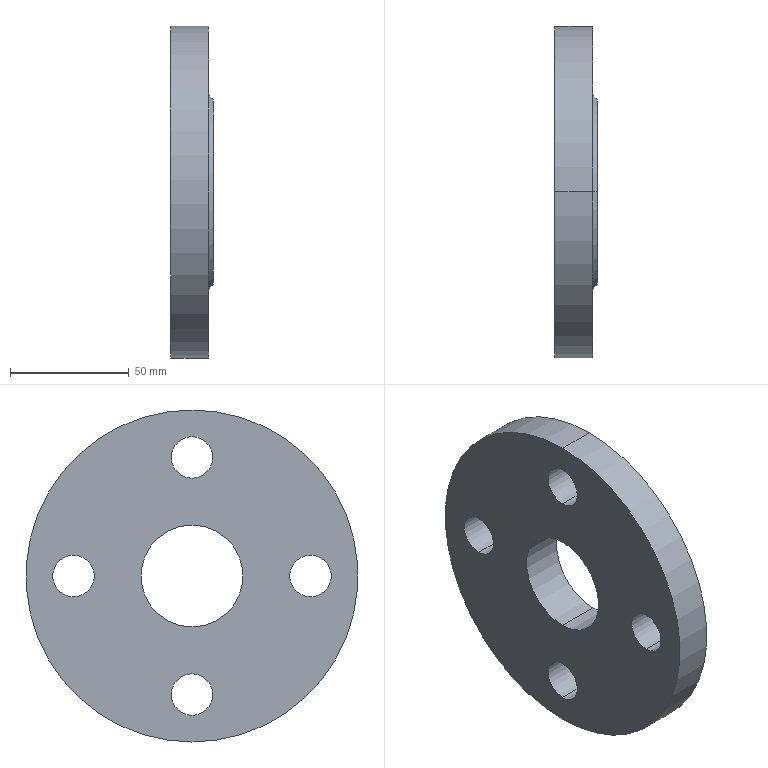Part | SolidWorks | features ICE 1, Revolution 1 | 1 solid | 17 faces | box 18 x 140 x 140 mm | volume 214823 mm3 | cylinder 12 | plane 3 | cone 2 | commonest cylinder face diameters 17.5 x8 43 x2 140 x2
STEP:
#1=CARTESIAN_POINT('',(0.,50.,8.75));
#2=VERTEX_POINT('',#1);
#3=CARTESIAN_POINT('',(0.,50.,-8.75));
#4=VERTEX_POINT('',#3);
#5=CARTESIAN_POINT('',(0.,50.,0.));
#6=DIRECTION('',(1.,0.,0.));
#7=DIRECTION('',(0.,0.,-1.));
#8=AXIS2_PLACEMENT_3D('',#5,#6,#7);
#9=CIRCLE('',#8,8.75);
#10=EDGE_CURVE('',#2,#4,#9,.T.);
#11=ORIENTED_EDGE('',*,*,#10,.F.);
#12=CARTESIAN_POINT('',(16.,50.,8.75));
#13=VERTEX_POINT('',#12);
#14=CARTESIAN_POINT('',(0.,50.,8.75));
#15=DIRECTION('',(1.,0.,0.));
#16=VECTOR('',#15,1000.);
#17=LINE('',#14,#16);
#18=EDGE_CURVE('',#2,#13,#17,.T.);
#19=ORIENTED_EDGE('',*,*,#18,.T.);
#20=CARTESIAN_POINT('',(16.,50.,-8.75));
#21=VERTEX_POINT('',#20);
#22=CARTESIAN_POINT('',(16.,50.,0.));
#23=DIRECTION('',(-1.,0.,0.));
#24=DIRECTION('',(0.,0.,1.));
#25=AXIS2_PLACEMENT_3D('',#22,#23,#24);
#26=CIRCLE('',#25,8.75);
#27=EDGE_CURVE('',#21,#13,#26,.T.);
#28=ORIENTED_EDGE('',*,*,#27,.F.);
#29=CARTESIAN_POINT('',(0.,50.,-8.75));
#30=DIRECTION('',(1.,0.,0.));
#31=VECTOR('',#30,1000.);
#32=LINE('',#29,#31);
#33=EDGE_CURVE('',#4,#21,#32,.T.);
#34=ORIENTED_EDGE('',*,*,#33,.F.);
#35=EDGE_LOOP('',(#11,#19,#28,#34));
#36=FACE_OUTER_BOUND('',#35,.T.);
#37=CARTESIAN_POINT('',(0.,50.,0.));
#38=DIRECTION('',(1.,0.,0.));
#39=DIRECTION('',(0.,0.,-1.));
#40=AXIS2_PLACEMENT_3D('',#37,#38,#39);
#41=CYLINDRICAL_SURFACE('',#40,8.75);
#42=ADVANCED_FACE('',(#36),#41,.F.);
#43=CARTESIAN_POINT('',(0.,0.,-41.25));
#44=VERTEX_POINT('',#43);
#45=CARTESIAN_POINT('',(0.,0.,-58.75));
#46=VERTEX_POINT('',#45);
#47=CARTESIAN_POINT('',(0.,0.,-50.));
#48=DIRECTION('',(1.,0.,0.));
#49=DIRECTION('',(0.,0.,-1.));
#50=AXIS2_PLACEMENT_3D('',#47,#48,#49);
#51=CIRCLE('',#50,8.75);
#52=EDGE_CURVE('',#44,#46,#51,.T.);
#53=ORIENTED_EDGE('',*,*,#52,.F.);
#54=CARTESIAN_POINT('',(16.,0.,-41.25));
#55=VERTEX_POINT('',#54);
#56=CARTESIAN_POINT('',(0.,0.,-41.25));
#57=DIRECTION('',(1.,0.,0.));
#58=VECTOR('',#57,1000.);
#59=LINE('',#56,#58);
#60=EDGE_CURVE('',#44,#55,#59,.T.);
#61=ORIENTED_EDGE('',*,*,#60,.T.);
#62=CARTESIAN_POINT('',(16.,0.,-58.75));
#63=VERTEX_POINT('',#62);
#64=CARTESIAN_POINT('',(16.,0.,-50.));
#65=DIRECTION('',(-1.,0.,0.));
#66=DIRECTION('',(0.,0.,1.));
#67=AXIS2_PLACEMENT_3D('',#64,#65,#66);
#68=CIRCLE('',#67,8.75);
#69=EDGE_CURVE('',#63,#55,#68,.T.);
#70=ORIENTED_EDGE('',*,*,#69,.F.);
#71=CARTESIAN_POINT('',(0.,0.,-58.75));
#72=DIRECTION('',(1.,0.,0.));
#73=VECTOR('',#72,1000.);
#74=LINE('',#71,#73);
#75=EDGE_CURVE('',#46,#63,#74,.T.);
#76=ORIENTED_EDGE('',*,*,#75,.F.);
#77=EDGE_LOOP('',(#53,#61,#70,#76));
#78=FACE_OUTER_BOUND('',#77,.T.);
#79=CARTESIAN_POINT('',(0.,0.,-50.));
#80=DIRECTION('',(1.,0.,0.));
#81=DIRECTION('',(0.,0.,-1.));
#82=AXIS2_PLACEMENT_3D('',#79,#80,#81);
#83=CYLINDRICAL_SURFACE('',#82,8.75);
#84=ADVANCED_FACE('',(#78),#83,.F.);
#85=CARTESIAN_POINT('',(0.,-50.,8.75));
#86=VERTEX_POINT('',#85);
#87=CARTESIAN_POINT('',(0.,-50.,-8.75));
#88=VERTEX_POINT('',#87);
#89=CARTESIAN_POINT('',(0.,-50.,0.));
#90=DIRECTION('',(1.,0.,0.));
#91=DIRECTION('',(0.,0.,-1.));
#92=AXIS2_PLACEMENT_3D('',#89,#90,#91);
#93=CIRCLE('',#92,8.75);
#94=EDGE_CURVE('',#86,#88,#93,.T.);
#95=ORIENTED_EDGE('',*,*,#94,.F.);
#96=CARTESIAN_POINT('',(16.,-50.,8.75));
#97=VERTEX_POINT('',#96);
#98=CARTESIAN_POINT('',(0.,-50.,8.75));
#99=DIRECTION('',(1.,0.,0.));
#100=VECTOR('',#99,1000.);
#101=LINE('',#98,#100);
#102=EDGE_CURVE('',#86,#97,#101,.T.);
#103=ORIENTED_EDGE('',*,*,#102,.T.);
#104=CARTESIAN_POINT('',(16.,-50.,-8.75));
#105=VERTEX_POINT('',#104);
#106=CARTESIAN_POINT('',(16.,-50.,0.));
#107=DIRECTION('',(-1.,0.,0.));
#108=DIRECTION('',(0.,0.,1.));
#109=AXIS2_PLACEMENT_3D('',#106,#107,#108);
#110=CIRCLE('',#109,8.75);
#111=EDGE_CURVE('',#105,#97,#110,.T.);
#112=ORIENTED_EDGE('',*,*,#111,.F.);
#113=CARTESIAN_POINT('',(0.,-50.,-8.75));
#114=DIRECTION('',(1.,0.,0.));
#115=VECTOR('',#114,1000.);
#116=LINE('',#113,#115);
#117=EDGE_CURVE('',#88,#105,#116,.T.);
#118=ORIENTED_EDGE('',*,*,#117,.F.);
#119=EDGE_LOOP('',(#95,#103,#112,#118));
#120=FACE_OUTER_BOUND('',#119,.T.);
#121=CARTESIAN_POINT('',(0.,-50.,0.));
#122=DIRECTION('',(1.,0.,0.));
#123=DIRECTION('',(0.,0.,-1.));
#124=AXIS2_PLACEMENT_3D('',#121,#122,#123);
#125=CYLINDRICAL_SURFACE('',#124,8.75);
#126=ADVANCED_FACE('',(#120),#125,.F.);
#127=CARTESIAN_POINT('',(0.,0.,58.75));
#128=VERTEX_POINT('',#127);
#129=CARTESIAN_POINT('',(0.,0.,41.25));
#130=VERTEX_POINT('',#129);
#131=CARTESIAN_POINT('',(0.,0.,50.));
#132=DIRECTION('',(1.,0.,0.));
#133=DIRECTION('',(0.,0.,-1.));
#134=AXIS2_PLACEMENT_3D('',#131,#132,#133);
#135=CIRCLE('',#134,8.75);
#136=EDGE_CURVE('',#128,#130,#135,.T.);
#137=ORIENTED_EDGE('',*,*,#136,.F.);
#138=CARTESIAN_POINT('',(16.,0.,58.75));
#139=VERTEX_POINT('',#138);
#140=CARTESIAN_POINT('',(0.,0.,58.75));
#141=DIRECTION('',(1.,0.,0.));
#142=VECTOR('',#141,1000.);
#143=LINE('',#140,#142);
#144=EDGE_CURVE('',#128,#139,#143,.T.);
#145=ORIENTED_EDGE('',*,*,#144,.T.);
#146=CARTESIAN_POINT('',(16.,0.,41.25));
#147=VERTEX_POINT('',#146);
#148=CARTESIAN_POINT('',(16.,0.,50.));
#149=DIRECTION('',(-1.,0.,0.));
#150=DIRECTION('',(0.,0.,1.));
#151=AXIS2_PLACEMENT_3D('',#148,#149,#150);
#152=CIRCLE('',#151,8.75);
#153=EDGE_CURVE('',#147,#139,#152,.T.);
#154=ORIENTED_EDGE('',*,*,#153,.F.);
#155=CARTESIAN_POINT('',(0.,0.,41.25));
#156=DIRECTION('',(1.,0.,0.));
#157=VECTOR('',#156,1000.);
#158=LINE('',#155,#157);
#159=EDGE_CURVE('',#130,#147,#158,.T.);
#160=ORIENTED_EDGE('',*,*,#159,.F.);
#161=EDGE_LOOP('',(#137,#145,#154,#160));
#162=FACE_OUTER_BOUND('',#161,.T.);
#163=CARTESIAN_POINT('',(0.,0.,50.));
#164=DIRECTION('',(1.,0.,0.));
#165=DIRECTION('',(0.,0.,-1.));
#166=AXIS2_PLACEMENT_3D('',#163,#164,#165);
#167=CYLINDRICAL_SURFACE('',#166,8.75);
#168=ADVANCED_FACE('',(#162),#167,.F.);
#169=CARTESIAN_POINT('',(18.,0.,39.));
#170=VERTEX_POINT('',#169);
#171=CARTESIAN_POINT('',(18.,0.,-39.));
#172=VERTEX_POINT('',#171);
#173=CARTESIAN_POINT('',(18.,0.,0.));
#174=DIRECTION('',(-1.,0.,0.));
#175=DIRECTION('',(0.,0.,1.));
#176=AXIS2_PLACEMENT_3D('',#173,#174,#175);
#177=CIRCLE('',#176,39.);
#178=EDGE_CURVE('',#170,#172,#177,.T.);
#179=ORIENTED_EDGE('',*,*,#178,.T.);
#180=CARTESIAN_POINT('',(16.,0.,-41.));
#181=VERTEX_POINT('',#180);
#182=CARTESIAN_POINT('',(18.,0.,-39.));
#183=DIRECTION('',(-0.7071,0.,-0.7071));
#184=VECTOR('',#183,1000.);
#185=LINE('',#182,#184);
#186=EDGE_CURVE('',#172,#181,#185,.T.);
#187=ORIENTED_EDGE('',*,*,#186,.T.);
#188=CARTESIAN_POINT('',(16.,0.,41.));
#189=VERTEX_POINT('',#188);
#190=CARTESIAN_POINT('',(16.,0.,0.));
#191=DIRECTION('',(-1.,0.,0.));
#192=DIRECTION('',(0.,0.,1.));
#193=AXIS2_PLACEMENT_3D('',#190,#191,#192);
#194=CIRCLE('',#193,41.);
#195=EDGE_CURVE('',#189,#181,#194,.T.);
#196=ORIENTED_EDGE('',*,*,#195,.F.);
#197=CARTESIAN_POINT('',(18.,0.,39.));
#198=DIRECTION('',(-0.7071,0.,0.7071));
#199=VECTOR('',#198,1000.);
#200=LINE('',#197,#199);
#201=EDGE_CURVE('',#170,#189,#200,.T.);
#202=ORIENTED_EDGE('',*,*,#201,.F.);
#203=EDGE_LOOP('',(#179,#187,#196,#202));
#204=FACE_OUTER_BOUND('',#203,.T.);
#205=CARTESIAN_POINT('',(18.,0.,0.));
#206=DIRECTION('',(-1.,0.,0.));
#207=DIRECTION('',(0.,0.,1.));
#208=AXIS2_PLACEMENT_3D('',#205,#206,#207);
#209=CONICAL_SURFACE('',#208,39.,0.7854);
#210=ADVANCED_FACE('',(#204),#209,.T.);
#211=CARTESIAN_POINT('',(16.,0.,70.));
#212=VERTEX_POINT('',#211);
#213=CARTESIAN_POINT('',(16.,0.,-70.));
#214=VERTEX_POINT('',#213);
#215=CARTESIAN_POINT('',(16.,0.,0.));
#216=DIRECTION('',(-1.,0.,0.));
#217=DIRECTION('',(0.,0.,1.));
#218=AXIS2_PLACEMENT_3D('',#215,#216,#217);
#219=CIRCLE('',#218,70.);
#220=EDGE_CURVE('',#212,#214,#219,.T.);
#221=ORIENTED_EDGE('',*,*,#220,.T.);
#222=CARTESIAN_POINT('',(0.,0.,-70.));
#223=VERTEX_POINT('',#222);
#224=CARTESIAN_POINT('',(0.,0.,-70.));
#225=DIRECTION('',(-1.,0.,0.));
#226=VECTOR('',#225,1000.);
#227=LINE('',#224,#226);
#228=EDGE_CURVE('',#214,#223,#227,.T.);
#229=ORIENTED_EDGE('',*,*,#228,.T.);
#230=CARTESIAN_POINT('',(0.,0.,70.));
#231=VERTEX_POINT('',#230);
#232=CARTESIAN_POINT('',(0.,0.,0.));
#233=DIRECTION('',(-1.,0.,0.));
#234=DIRECTION('',(0.,0.,1.));
#235=AXIS2_PLACEMENT_3D('',#232,#233,#234);
#236=CIRCLE('',#235,70.);
#237=EDGE_CURVE('',#231,#223,#236,.T.);
#238=ORIENTED_EDGE('',*,*,#237,.F.);
#239=CARTESIAN_POINT('',(0.,0.,70.));
#240=DIRECTION('',(-1.,0.,0.));
#241=VECTOR('',#240,1000.);
#242=LINE('',#239,#241);
#243=EDGE_CURVE('',#212,#231,#242,.T.);
#244=ORIENTED_EDGE('',*,*,#243,.F.);
#245=EDGE_LOOP('',(#221,#229,#238,#244));
#246=FACE_OUTER_BOUND('',#245,.T.);
#247=CARTESIAN_POINT('',(0.,0.,0.));
#248=DIRECTION('',(-1.,0.,0.));
#249=DIRECTION('',(0.,0.,1.));
#250=AXIS2_PLACEMENT_3D('',#247,#248,#249);
#251=CYLINDRICAL_SURFACE('',#250,70.);
#252=ADVANCED_FACE('',(#246),#251,.T.);
#253=CARTESIAN_POINT('',(18.,0.,-21.5));
#254=VERTEX_POINT('',#253);
#255=CARTESIAN_POINT('',(18.,0.,21.5));
#256=VERTEX_POINT('',#255);
#257=CARTESIAN_POINT('',(18.,0.,0.));
#258=DIRECTION('',(-1.,0.,0.));
#259=DIRECTION('',(0.,0.,1.));
#260=AXIS2_PLACEMENT_3D('',#257,#258,#259);
#261=CIRCLE('',#260,21.5);
#262=EDGE_CURVE('',#254,#256,#261,.T.);
#263=ORIENTED_EDGE('',*,*,#262,.F.);
#264=CARTESIAN_POINT('',(0.,0.,-21.5));
#265=VERTEX_POINT('',#264);
#266=CARTESIAN_POINT('',(0.,0.,-21.5));
#267=DIRECTION('',(-1.,0.,0.));
#268=VECTOR('',#267,1000.);
#269=LINE('',#266,#268);
#270=EDGE_CURVE('',#254,#265,#269,.T.);
#271=ORIENTED_EDGE('',*,*,#270,.T.);
#272=CARTESIAN_POINT('',(0.,0.,21.5));
#273=VERTEX_POINT('',#272);
#274=CARTESIAN_POINT('',(0.,0.,0.));
#275=DIRECTION('',(-1.,0.,0.));
#276=DIRECTION('',(0.,0.,1.));
#277=AXIS2_PLACEMENT_3D('',#274,#275,#276);
#278=CIRCLE('',#277,21.5);
#279=EDGE_CURVE('',#265,#273,#278,.T.);
#280=ORIENTED_EDGE('',*,*,#279,.T.);
#281=CARTESIAN_POINT('',(0.,0.,21.5));
#282=DIRECTION('',(-1.,0.,0.));
#283=VECTOR('',#282,1000.);
#284=LINE('',#281,#283);
#285=EDGE_CURVE('',#256,#273,#284,.T.);
#286=ORIENTED_EDGE('',*,*,#285,.F.);
#287=EDGE_LOOP('',(#263,#271,#280,#286));
#288=FACE_OUTER_BOUND('',#287,.T.);
#289=CARTESIAN_POINT('',(0.,0.,0.));
#290=DIRECTION('',(-1.,0.,0.));
#291=DIRECTION('',(0.,0.,1.));
#292=AXIS2_PLACEMENT_3D('',#289,#290,#291);
#293=CYLINDRICAL_SURFACE('',#292,21.5);
#294=ADVANCED_FACE('',(#288),#293,.F.);
#295=ORIENTED_EDGE('',*,*,#270,.F.);
#296=CARTESIAN_POINT('',(18.,0.,0.));
#297=DIRECTION('',(-1.,0.,0.));
#298=DIRECTION('',(0.,0.,1.));
#299=AXIS2_PLACEMENT_3D('',#296,#297,#298);
#300=CIRCLE('',#299,21.5);
#301=EDGE_CURVE('',#256,#254,#300,.T.);
#302=ORIENTED_EDGE('',*,*,#301,.F.);
#303=ORIENTED_EDGE('',*,*,#285,.T.);
#304=CARTESIAN_POINT('',(0.,0.,0.));
#305=DIRECTION('',(-1.,0.,0.));
#306=DIRECTION('',(0.,0.,1.));
#307=AXIS2_PLACEMENT_3D('',#304,#305,#306);
#308=CIRCLE('',#307,21.5);
#309=EDGE_CURVE('',#273,#265,#308,.T.);
#310=ORIENTED_EDGE('',*,*,#309,.T.);
#311=EDGE_LOOP('',(#295,#302,#303,#310));
#312=FACE_OUTER_BOUND('',#311,.T.);
#313=CARTESIAN_POINT('',(0.,0.,0.));
#314=DIRECTION('',(-1.,0.,0.));
#315=DIRECTION('',(0.,0.,1.));
#316=AXIS2_PLACEMENT_3D('',#313,#314,#315);
#317=CYLINDRICAL_SURFACE('',#316,21.5);
#318=ADVANCED_FACE('',(#312),#317,.F.);
#319=CARTESIAN_POINT('',(0.,50.,0.));
#320=DIRECTION('',(1.,0.,0.));
#321=DIRECTION('',(0.,0.,-1.));
#322=AXIS2_PLACEMENT_3D('',#319,#320,#321);
#323=CIRCLE('',#322,8.75);
#324=EDGE_CURVE('',#4,#2,#323,.T.);
#325=ORIENTED_EDGE('',*,*,#324,.T.);
#326=ORIENTED_EDGE('',*,*,#10,.T.);
#327=EDGE_LOOP('',(#325,#326));
#328=FACE_BOUND('',#327,.T.);
#329=CARTESIAN_POINT('',(0.,0.,-50.));
#330=DIRECTION('',(1.,0.,0.));
#331=DIRECTION('',(0.,0.,-1.));
#332=AXIS2_PLACEMENT_3D('',#329,#330,#331);
#333=CIRCLE('',#332,8.75);
#334=EDGE_CURVE('',#46,#44,#333,.T.);
#335=ORIENTED_EDGE('',*,*,#334,.T.);
#336=ORIENTED_EDGE('',*,*,#52,.T.);
#337=EDGE_LOOP('',(#335,#336));
#338=FACE_BOUND('',#337,.T.);
#339=CARTESIAN_POINT('',(0.,-50.,0.));
#340=DIRECTION('',(1.,0.,0.));
#341=DIRECTION('',(0.,0.,-1.));
#342=AXIS2_PLACEMENT_3D('',#339,#340,#341);
#343=CIRCLE('',#342,8.75);
#344=EDGE_CURVE('',#88,#86,#343,.T.);
#345=ORIENTED_EDGE('',*,*,#344,.T.);
#346=ORIENTED_EDGE('',*,*,#94,.T.);
#347=EDGE_LOOP('',(#345,#346));
#348=FACE_BOUND('',#347,.T.);
#349=CARTESIAN_POINT('',(0.,0.,50.));
#350=DIRECTION('',(1.,0.,0.));
#351=DIRECTION('',(0.,0.,-1.));
#352=AXIS2_PLACEMENT_3D('',#349,#350,#351);
#353=CIRCLE('',#352,8.75);
#354=EDGE_CURVE('',#130,#128,#353,.T.);
#355=ORIENTED_EDGE('',*,*,#354,.T.);
#356=ORIENTED_EDGE('',*,*,#136,.T.);
#357=EDGE_LOOP('',(#355,#356));
#358=FACE_BOUND('',#357,.T.);
#359=ORIENTED_EDGE('',*,*,#309,.F.);
#360=ORIENTED_EDGE('',*,*,#279,.F.);
#361=EDGE_LOOP('',(#359,#360));
#362=FACE_BOUND('',#361,.T.);
#363=ORIENTED_EDGE('',*,*,#237,.T.);
#364=CARTESIAN_POINT('',(0.,0.,0.));
#365=DIRECTION('',(-1.,0.,0.));
#366=DIRECTION('',(0.,0.,1.));
#367=AXIS2_PLACEMENT_3D('',#364,#365,#366);
#368=CIRCLE('',#367,70.);
#369=EDGE_CURVE('',#223,#231,#368,.T.);
#370=ORIENTED_EDGE('',*,*,#369,.T.);
#371=EDGE_LOOP('',(#363,#370));
#372=FACE_OUTER_BOUND('',#371,.T.);
#373=CARTESIAN_POINT('',(0.,0.,-21.5));
#374=DIRECTION('',(1.,0.,0.));
#375=DIRECTION('',(0.,0.,-1.));
#376=AXIS2_PLACEMENT_3D('',#373,#374,#375);
#377=PLANE('',#376);
#378=ADVANCED_FACE('',(#328,#338,#348,#358,#362,#372),#377,.F.);
#379=ORIENTED_EDGE('',*,*,#228,.F.);
#380=CARTESIAN_POINT('',(16.,0.,0.));
#381=DIRECTION('',(-1.,0.,0.));
#382=DIRECTION('',(0.,0.,1.));
#383=AXIS2_PLACEMENT_3D('',#380,#381,#382);
#384=CIRCLE('',#383,70.);
#385=EDGE_CURVE('',#214,#212,#384,.T.);
#386=ORIENTED_EDGE('',*,*,#385,.T.);
#387=ORIENTED_EDGE('',*,*,#243,.T.);
#388=ORIENTED_EDGE('',*,*,#369,.F.);
#389=EDGE_LOOP('',(#379,#386,#387,#388));
#390=FACE_OUTER_BOUND('',#389,.T.);
#391=CARTESIAN_POINT('',(0.,0.,0.));
#392=DIRECTION('',(-1.,0.,0.));
#393=DIRECTION('',(0.,0.,1.));
#394=AXIS2_PLACEMENT_3D('',#391,#392,#393);
#395=CYLINDRICAL_SURFACE('',#394,70.);
#396=ADVANCED_FACE('',(#390),#395,.T.);
#397=ORIENTED_EDGE('',*,*,#27,.T.);
#398=CARTESIAN_POINT('',(16.,50.,0.));
#399=DIRECTION('',(-1.,0.,0.));
#400=DIRECTION('',(0.,0.,1.));
#401=AXIS2_PLACEMENT_3D('',#398,#399,#400);
#402=CIRCLE('',#401,8.75);
#403=EDGE_CURVE('',#13,#21,#402,.T.);
#404=ORIENTED_EDGE('',*,*,#403,.T.);
#405=EDGE_LOOP('',(#397,#404));
#406=FACE_BOUND('',#405,.T.);
#407=ORIENTED_EDGE('',*,*,#69,.T.);
#408=CARTESIAN_POINT('',(16.,0.,-50.));
#409=DIRECTION('',(-1.,0.,0.));
#410=DIRECTION('',(0.,0.,1.));
#411=AXIS2_PLACEMENT_3D('',#408,#409,#410);
#412=CIRCLE('',#411,8.75);
#413=EDGE_CURVE('',#55,#63,#412,.T.);
#414=ORIENTED_EDGE('',*,*,#413,.T.);
#415=EDGE_LOOP('',(#407,#414));
#416=FACE_BOUND('',#415,.T.);
#417=ORIENTED_EDGE('',*,*,#111,.T.);
#418=CARTESIAN_POINT('',(16.,-50.,0.));
#419=DIRECTION('',(-1.,0.,0.));
#420=DIRECTION('',(0.,0.,1.));
#421=AXIS2_PLACEMENT_3D('',#418,#419,#420);
#422=CIRCLE('',#421,8.75);
#423=EDGE_CURVE('',#97,#105,#422,.T.);
#424=ORIENTED_EDGE('',*,*,#423,.T.);
#425=EDGE_LOOP('',(#417,#424));
#426=FACE_BOUND('',#425,.T.);
#427=ORIENTED_EDGE('',*,*,#153,.T.);
#428=CARTESIAN_POINT('',(16.,0.,50.));
#429=DIRECTION('',(-1.,0.,0.));
#430=DIRECTION('',(0.,0.,1.));
#431=AXIS2_PLACEMENT_3D('',#428,#429,#430);
#432=CIRCLE('',#431,8.75);
#433=EDGE_CURVE('',#139,#147,#432,.T.);
#434=ORIENTED_EDGE('',*,*,#433,.T.);
#435=EDGE_LOOP('',(#427,#434));
#436=FACE_BOUND('',#435,.T.);
#437=ORIENTED_EDGE('',*,*,#220,.F.);
#438=ORIENTED_EDGE('',*,*,#385,.F.);
#439=EDGE_LOOP('',(#437,#438));
#440=FACE_OUTER_BOUND('',#439,.T.);
#441=ORIENTED_EDGE('',*,*,#195,.T.);
#442=CARTESIAN_POINT('',(16.,0.,0.));
#443=DIRECTION('',(-1.,0.,0.));
#444=DIRECTION('',(0.,0.,1.));
#445=AXIS2_PLACEMENT_3D('',#442,#443,#444);
#446=CIRCLE('',#445,41.);
#447=EDGE_CURVE('',#181,#189,#446,.T.);
#448=ORIENTED_EDGE('',*,*,#447,.T.);
#449=EDGE_LOOP('',(#441,#448));
#450=FACE_BOUND('',#449,.T.);
#451=CARTESIAN_POINT('',(16.,0.,-70.));
#452=DIRECTION('',(-1.,0.,0.));
#453=DIRECTION('',(0.,0.,1.));
#454=AXIS2_PLACEMENT_3D('',#451,#452,#453);
#455=PLANE('',#454);
#456=ADVANCED_FACE('',(#406,#416,#426,#436,#440,#450),#455,.F.);
#457=ORIENTED_EDGE('',*,*,#186,.F.);
#458=CARTESIAN_POINT('',(18.,0.,0.));
#459=DIRECTION('',(-1.,0.,0.));
#460=DIRECTION('',(0.,0.,1.));
#461=AXIS2_PLACEMENT_3D('',#458,#459,#460);
#462=CIRCLE('',#461,39.);
#463=EDGE_CURVE('',#172,#170,#462,.T.);
#464=ORIENTED_EDGE('',*,*,#463,.T.);
#465=ORIENTED_EDGE('',*,*,#201,.T.);
#466=ORIENTED_EDGE('',*,*,#447,.F.);
#467=EDGE_LOOP('',(#457,#464,#465,#466));
#468=FACE_OUTER_BOUND('',#467,.T.);
#469=CARTESIAN_POINT('',(18.,0.,0.));
#470=DIRECTION('',(-1.,0.,0.));
#471=DIRECTION('',(0.,0.,1.));
#472=AXIS2_PLACEMENT_3D('',#469,#470,#471);
#473=CONICAL_SURFACE('',#472,39.,0.7854);
#474=ADVANCED_FACE('',(#468),#473,.T.);
#475=ORIENTED_EDGE('',*,*,#178,.F.);
#476=ORIENTED_EDGE('',*,*,#463,.F.);
#477=EDGE_LOOP('',(#475,#476));
#478=FACE_OUTER_BOUND('',#477,.T.);
#479=ORIENTED_EDGE('',*,*,#301,.T.);
#480=ORIENTED_EDGE('',*,*,#262,.T.);
#481=EDGE_LOOP('',(#479,#480));
#482=FACE_BOUND('',#481,.T.);
#483=CARTESIAN_POINT('',(18.,0.,-39.));
#484=DIRECTION('',(-1.,0.,0.));
#485=DIRECTION('',(0.,0.,1.));
#486=AXIS2_PLACEMENT_3D('',#483,#484,#485);
#487=PLANE('',#486);
#488=ADVANCED_FACE('',(#478,#482),#487,.F.);
#489=ORIENTED_EDGE('',*,*,#144,.F.);
#490=ORIENTED_EDGE('',*,*,#354,.F.);
#491=ORIENTED_EDGE('',*,*,#159,.T.);
#492=ORIENTED_EDGE('',*,*,#433,.F.);
#493=EDGE_LOOP('',(#489,#490,#491,#492));
#494=FACE_OUTER_BOUND('',#493,.T.);
#495=CARTESIAN_POINT('',(0.,0.,50.));
#496=DIRECTION('',(1.,0.,0.));
#497=DIRECTION('',(0.,0.,-1.));
#498=AXIS2_PLACEMENT_3D('',#495,#496,#497);
#499=CYLINDRICAL_SURFACE('',#498,8.75);
#500=ADVANCED_FACE('',(#494),#499,.F.);
#501=ORIENTED_EDGE('',*,*,#102,.F.);
#502=ORIENTED_EDGE('',*,*,#344,.F.);
#503=ORIENTED_EDGE('',*,*,#117,.T.);
#504=ORIENTED_EDGE('',*,*,#423,.F.);
#505=EDGE_LOOP('',(#501,#502,#503,#504));
#506=FACE_OUTER_BOUND('',#505,.T.);
#507=CARTESIAN_POINT('',(0.,-50.,0.));
#508=DIRECTION('',(1.,0.,0.));
#509=DIRECTION('',(0.,0.,-1.));
#510=AXIS2_PLACEMENT_3D('',#507,#508,#509);
#511=CYLINDRICAL_SURFACE('',#510,8.75);
#512=ADVANCED_FACE('',(#506),#511,.F.);
#513=ORIENTED_EDGE('',*,*,#60,.F.);
#514=ORIENTED_EDGE('',*,*,#334,.F.);
#515=ORIENTED_EDGE('',*,*,#75,.T.);
#516=ORIENTED_EDGE('',*,*,#413,.F.);
#517=EDGE_LOOP('',(#513,#514,#515,#516));
#518=FACE_OUTER_BOUND('',#517,.T.);
#519=CARTESIAN_POINT('',(0.,0.,-50.));
#520=DIRECTION('',(1.,0.,0.));
#521=DIRECTION('',(0.,0.,-1.));
#522=AXIS2_PLACEMENT_3D('',#519,#520,#521);
#523=CYLINDRICAL_SURFACE('',#522,8.75);
#524=ADVANCED_FACE('',(#518),#523,.F.);
#525=ORIENTED_EDGE('',*,*,#18,.F.);
#526=ORIENTED_EDGE('',*,*,#324,.F.);
#527=ORIENTED_EDGE('',*,*,#33,.T.);
#528=ORIENTED_EDGE('',*,*,#403,.F.);
#529=EDGE_LOOP('',(#525,#526,#527,#528));
#530=FACE_OUTER_BOUND('',#529,.T.);
#531=CARTESIAN_POINT('',(0.,50.,0.));
#532=DIRECTION('',(1.,0.,0.));
#533=DIRECTION('',(0.,0.,-1.));
#534=AXIS2_PLACEMENT_3D('',#531,#532,#533);
#535=CYLINDRICAL_SURFACE('',#534,8.75);
#536=ADVANCED_FACE('',(#530),#535,.F.);
#537=CLOSED_SHELL('',(#42,#84,#126,#168,#210,#252,#294,#318,#378,#396,#456,#474,#488,#500,#512,#524,#536));
#538=MANIFOLD_SOLID_BREP('',#537);
#539=CARTESIAN_POINT('',(0.,0.,0.));
#540=DIRECTION('',(0.,0.,1.));
#541=DIRECTION('',(1.,0.,0.));
#542=AXIS2_PLACEMENT_3D('',#539,#540,#541);
#543=(LENGTH_UNIT()NAMED_UNIT(*)SI_UNIT(.MILLI.,.METRE.));
#544=UNCERTAINTY_MEASURE_WITH_UNIT(LENGTH_MEASURE(0.00001),#543,'','');
#545=(NAMED_UNIT(*)PLANE_ANGLE_UNIT()SI_UNIT($,.RADIAN.));
#546=(NAMED_UNIT(*)SI_UNIT($,.STERADIAN.)SOLID_ANGLE_UNIT());
#547=(GEOMETRIC_REPRESENTATION_CONTEXT(3)GLOBAL_UNCERTAINTY_ASSIGNED_CONTEXT((#544))GLOBAL_UNIT_ASSIGNED_CONTEXT((#543,#545,#546))REPRESENTATION_CONTEXT('',''));
#548=ADVANCED_BREP_SHAPE_REPRESENTATION('',(#538,#542),#547);